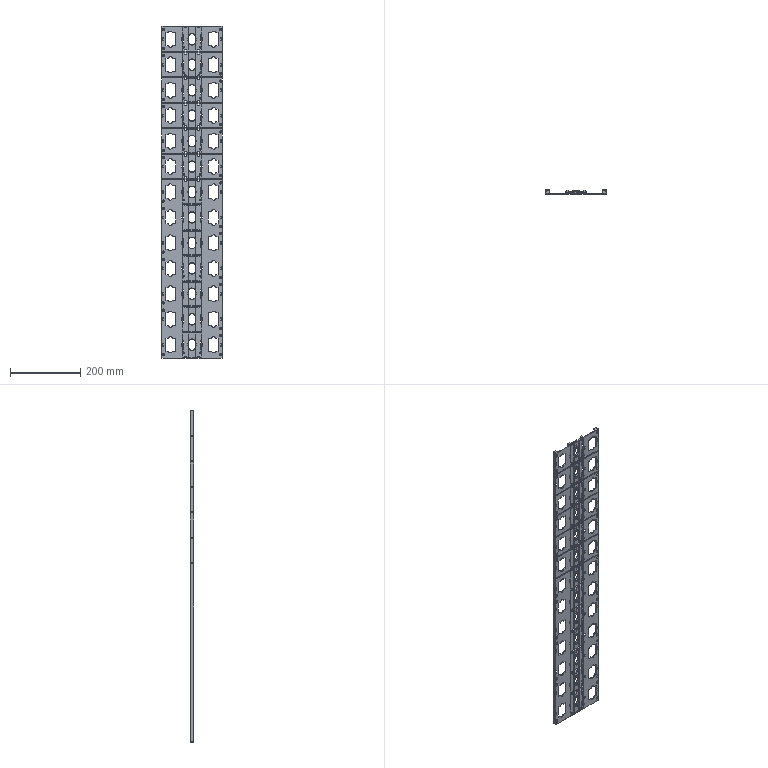Part | NX | features BREP 1 | 1 solid | 3806 faces | volume 265096 mm3 | plane 2312 | cylinder 1494 | commonest cylinder face diameters 2 x361 4 x240 3 x156 6 x104 3.2 x92 9 x84